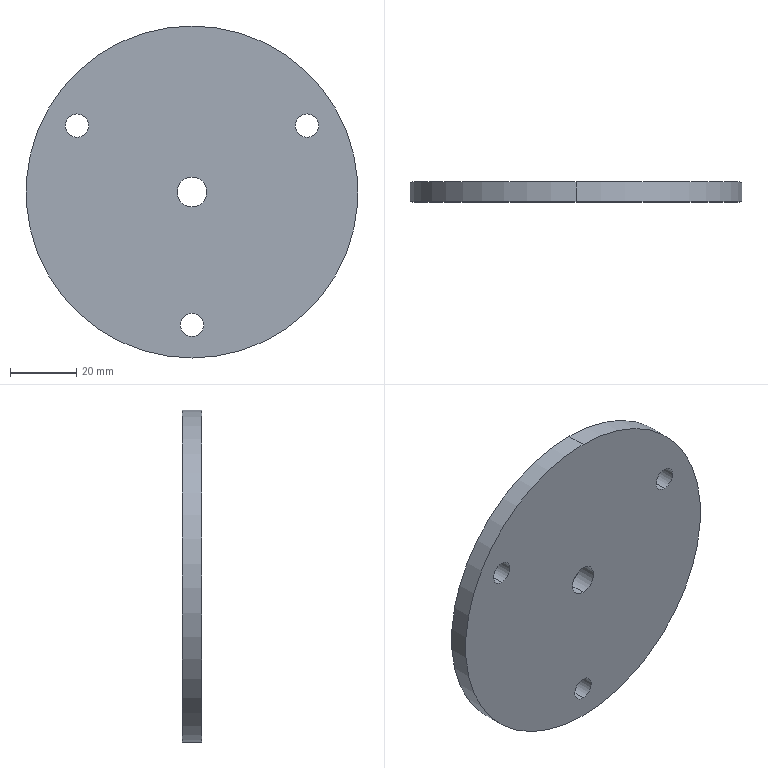Part | SolidWorks | features Extrusion 1, HoleWzd 1, ICE 1 | 1 solid | 12 faces | box 100 x 6 x 100 mm | volume 46049 mm3 | cylinder 10 | plane 2 | commonest cylinder face diameters 7 x6 9 x2 100 x2
STEP:
#1=CARTESIAN_POINT('',(0.,-3.,-4.5));
#2=VERTEX_POINT('',#1);
#3=CARTESIAN_POINT('',(0.,-3.,4.5));
#4=VERTEX_POINT('',#3);
#5=CARTESIAN_POINT('',(0.,-3.,0.));
#6=DIRECTION('',(0.,1.,0.));
#7=DIRECTION('',(0.,0.,1.));
#8=AXIS2_PLACEMENT_3D('',#5,#6,#7);
#9=CIRCLE('',#8,4.5);
#10=EDGE_CURVE('',#2,#4,#9,.T.);
#11=ORIENTED_EDGE('',*,*,#10,.F.);
#12=CARTESIAN_POINT('',(0.,3.,-4.5));
#13=VERTEX_POINT('',#12);
#14=CARTESIAN_POINT('',(0.,3.,-4.5));
#15=DIRECTION('',(0.,1.,0.));
#16=VECTOR('',#15,1000.);
#17=LINE('',#14,#16);
#18=EDGE_CURVE('',#2,#13,#17,.T.);
#19=ORIENTED_EDGE('',*,*,#18,.T.);
#20=CARTESIAN_POINT('',(0.,3.,4.5));
#21=VERTEX_POINT('',#20);
#22=CARTESIAN_POINT('',(0.,3.,0.));
#23=DIRECTION('',(0.,1.,0.));
#24=DIRECTION('',(0.,0.,1.));
#25=AXIS2_PLACEMENT_3D('',#22,#23,#24);
#26=CIRCLE('',#25,4.5);
#27=EDGE_CURVE('',#13,#21,#26,.T.);
#28=ORIENTED_EDGE('',*,*,#27,.T.);
#29=CARTESIAN_POINT('',(0.,3.,4.5));
#30=DIRECTION('',(0.,1.,0.));
#31=VECTOR('',#30,1000.);
#32=LINE('',#29,#31);
#33=EDGE_CURVE('',#4,#21,#32,.T.);
#34=ORIENTED_EDGE('',*,*,#33,.F.);
#35=EDGE_LOOP('',(#11,#19,#28,#34));
#36=FACE_OUTER_BOUND('',#35,.T.);
#37=CARTESIAN_POINT('',(0.,3.,0.));
#38=DIRECTION('',(0.,1.,0.));
#39=DIRECTION('',(0.,0.,1.));
#40=AXIS2_PLACEMENT_3D('',#37,#38,#39);
#41=CYLINDRICAL_SURFACE('',#40,4.5);
#42=ADVANCED_FACE('',(#36),#41,.F.);
#43=CARTESIAN_POINT('',(-34.641,-3.,16.5));
#44=VERTEX_POINT('',#43);
#45=CARTESIAN_POINT('',(-34.641,-3.,23.5));
#46=VERTEX_POINT('',#45);
#47=CARTESIAN_POINT('',(-34.641,-3.,20.));
#48=DIRECTION('',(0.,1.,0.));
#49=DIRECTION('',(0.,0.,1.));
#50=AXIS2_PLACEMENT_3D('',#47,#48,#49);
#51=CIRCLE('',#50,3.5);
#52=EDGE_CURVE('',#44,#46,#51,.T.);
#53=ORIENTED_EDGE('',*,*,#52,.F.);
#54=CARTESIAN_POINT('',(-34.641,3.,16.5));
#55=VERTEX_POINT('',#54);
#56=CARTESIAN_POINT('',(-34.641,-3.,16.5));
#57=DIRECTION('',(0.,1.,0.));
#58=VECTOR('',#57,1000.);
#59=LINE('',#56,#58);
#60=EDGE_CURVE('',#44,#55,#59,.T.);
#61=ORIENTED_EDGE('',*,*,#60,.T.);
#62=CARTESIAN_POINT('',(-34.641,3.,23.5));
#63=VERTEX_POINT('',#62);
#64=CARTESIAN_POINT('',(-34.641,3.,20.));
#65=DIRECTION('',(0.,1.,0.));
#66=DIRECTION('',(0.,0.,1.));
#67=AXIS2_PLACEMENT_3D('',#64,#65,#66);
#68=CIRCLE('',#67,3.5);
#69=EDGE_CURVE('',#55,#63,#68,.T.);
#70=ORIENTED_EDGE('',*,*,#69,.T.);
#71=CARTESIAN_POINT('',(-34.641,-3.,23.5));
#72=DIRECTION('',(0.,1.,0.));
#73=VECTOR('',#72,1000.);
#74=LINE('',#71,#73);
#75=EDGE_CURVE('',#46,#63,#74,.T.);
#76=ORIENTED_EDGE('',*,*,#75,.F.);
#77=EDGE_LOOP('',(#53,#61,#70,#76));
#78=FACE_OUTER_BOUND('',#77,.T.);
#79=CARTESIAN_POINT('',(-34.641,-3.,20.));
#80=DIRECTION('',(0.,1.,0.));
#81=DIRECTION('',(0.,0.,1.));
#82=AXIS2_PLACEMENT_3D('',#79,#80,#81);
#83=CYLINDRICAL_SURFACE('',#82,3.5);
#84=ADVANCED_FACE('',(#78),#83,.F.);
#85=CARTESIAN_POINT('',(34.641,-3.,16.5));
#86=VERTEX_POINT('',#85);
#87=CARTESIAN_POINT('',(34.641,-3.,23.5));
#88=VERTEX_POINT('',#87);
#89=CARTESIAN_POINT('',(34.641,-3.,20.));
#90=DIRECTION('',(0.,1.,0.));
#91=DIRECTION('',(0.,0.,1.));
#92=AXIS2_PLACEMENT_3D('',#89,#90,#91);
#93=CIRCLE('',#92,3.5);
#94=EDGE_CURVE('',#86,#88,#93,.T.);
#95=ORIENTED_EDGE('',*,*,#94,.F.);
#96=CARTESIAN_POINT('',(34.641,3.,16.5));
#97=VERTEX_POINT('',#96);
#98=CARTESIAN_POINT('',(34.641,-3.,16.5));
#99=DIRECTION('',(0.,1.,0.));
#100=VECTOR('',#99,1000.);
#101=LINE('',#98,#100);
#102=EDGE_CURVE('',#86,#97,#101,.T.);
#103=ORIENTED_EDGE('',*,*,#102,.T.);
#104=CARTESIAN_POINT('',(34.641,3.,23.5));
#105=VERTEX_POINT('',#104);
#106=CARTESIAN_POINT('',(34.641,3.,20.));
#107=DIRECTION('',(0.,1.,0.));
#108=DIRECTION('',(0.,0.,1.));
#109=AXIS2_PLACEMENT_3D('',#106,#107,#108);
#110=CIRCLE('',#109,3.5);
#111=EDGE_CURVE('',#97,#105,#110,.T.);
#112=ORIENTED_EDGE('',*,*,#111,.T.);
#113=CARTESIAN_POINT('',(34.641,-3.,23.5));
#114=DIRECTION('',(0.,1.,0.));
#115=VECTOR('',#114,1000.);
#116=LINE('',#113,#115);
#117=EDGE_CURVE('',#88,#105,#116,.T.);
#118=ORIENTED_EDGE('',*,*,#117,.F.);
#119=EDGE_LOOP('',(#95,#103,#112,#118));
#120=FACE_OUTER_BOUND('',#119,.T.);
#121=CARTESIAN_POINT('',(34.641,-3.,20.));
#122=DIRECTION('',(0.,1.,0.));
#123=DIRECTION('',(0.,0.,1.));
#124=AXIS2_PLACEMENT_3D('',#121,#122,#123);
#125=CYLINDRICAL_SURFACE('',#124,3.5);
#126=ADVANCED_FACE('',(#120),#125,.F.);
#127=CARTESIAN_POINT('',(0.,-3.,-43.5));
#128=VERTEX_POINT('',#127);
#129=CARTESIAN_POINT('',(0.,-3.,-36.5));
#130=VERTEX_POINT('',#129);
#131=CARTESIAN_POINT('',(0.,-3.,-40.));
#132=DIRECTION('',(0.,1.,0.));
#133=DIRECTION('',(0.,0.,1.));
#134=AXIS2_PLACEMENT_3D('',#131,#132,#133);
#135=CIRCLE('',#134,3.5);
#136=EDGE_CURVE('',#128,#130,#135,.T.);
#137=ORIENTED_EDGE('',*,*,#136,.F.);
#138=CARTESIAN_POINT('',(0.,3.,-43.5));
#139=VERTEX_POINT('',#138);
#140=CARTESIAN_POINT('',(0.,-3.,-43.5));
#141=DIRECTION('',(0.,1.,0.));
#142=VECTOR('',#141,1000.);
#143=LINE('',#140,#142);
#144=EDGE_CURVE('',#128,#139,#143,.T.);
#145=ORIENTED_EDGE('',*,*,#144,.T.);
#146=CARTESIAN_POINT('',(0.,3.,-36.5));
#147=VERTEX_POINT('',#146);
#148=CARTESIAN_POINT('',(0.,3.,-40.));
#149=DIRECTION('',(0.,1.,0.));
#150=DIRECTION('',(0.,0.,1.));
#151=AXIS2_PLACEMENT_3D('',#148,#149,#150);
#152=CIRCLE('',#151,3.5);
#153=EDGE_CURVE('',#139,#147,#152,.T.);
#154=ORIENTED_EDGE('',*,*,#153,.T.);
#155=CARTESIAN_POINT('',(0.,-3.,-36.5));
#156=DIRECTION('',(0.,1.,0.));
#157=VECTOR('',#156,1000.);
#158=LINE('',#155,#157);
#159=EDGE_CURVE('',#130,#147,#158,.T.);
#160=ORIENTED_EDGE('',*,*,#159,.F.);
#161=EDGE_LOOP('',(#137,#145,#154,#160));
#162=FACE_OUTER_BOUND('',#161,.T.);
#163=CARTESIAN_POINT('',(0.,-3.,-40.));
#164=DIRECTION('',(0.,1.,0.));
#165=DIRECTION('',(0.,0.,1.));
#166=AXIS2_PLACEMENT_3D('',#163,#164,#165);
#167=CYLINDRICAL_SURFACE('',#166,3.5);
#168=ADVANCED_FACE('',(#162),#167,.F.);
#169=CARTESIAN_POINT('',(0.,3.,50.));
#170=VERTEX_POINT('',#169);
#171=CARTESIAN_POINT('',(0.,3.,-50.));
#172=VERTEX_POINT('',#171);
#173=CARTESIAN_POINT('',(0.,3.,0.));
#174=DIRECTION('',(0.,1.,0.));
#175=DIRECTION('',(0.,0.,1.));
#176=AXIS2_PLACEMENT_3D('',#173,#174,#175);
#177=CIRCLE('',#176,50.);
#178=EDGE_CURVE('',#170,#172,#177,.T.);
#179=ORIENTED_EDGE('',*,*,#178,.F.);
#180=CARTESIAN_POINT('',(0.,-3.,50.));
#181=VERTEX_POINT('',#180);
#182=CARTESIAN_POINT('',(0.,3.,50.));
#183=DIRECTION('',(0.,-1.,0.));
#184=VECTOR('',#183,1000.);
#185=LINE('',#182,#184);
#186=EDGE_CURVE('',#170,#181,#185,.T.);
#187=ORIENTED_EDGE('',*,*,#186,.T.);
#188=CARTESIAN_POINT('',(0.,-3.,-50.));
#189=VERTEX_POINT('',#188);
#190=CARTESIAN_POINT('',(0.,-3.,0.));
#191=DIRECTION('',(0.,1.,0.));
#192=DIRECTION('',(0.,0.,1.));
#193=AXIS2_PLACEMENT_3D('',#190,#191,#192);
#194=CIRCLE('',#193,50.);
#195=EDGE_CURVE('',#181,#189,#194,.T.);
#196=ORIENTED_EDGE('',*,*,#195,.T.);
#197=CARTESIAN_POINT('',(0.,3.,-50.));
#198=DIRECTION('',(0.,-1.,0.));
#199=VECTOR('',#198,1000.);
#200=LINE('',#197,#199);
#201=EDGE_CURVE('',#172,#189,#200,.T.);
#202=ORIENTED_EDGE('',*,*,#201,.F.);
#203=EDGE_LOOP('',(#179,#187,#196,#202));
#204=FACE_OUTER_BOUND('',#203,.T.);
#205=CARTESIAN_POINT('',(0.,3.,0.));
#206=DIRECTION('',(0.,-1.,0.));
#207=DIRECTION('',(0.,0.,-1.));
#208=AXIS2_PLACEMENT_3D('',#205,#206,#207);
#209=CYLINDRICAL_SURFACE('',#208,50.);
#210=ADVANCED_FACE('',(#204),#209,.T.);
#211=ORIENTED_EDGE('',*,*,#186,.F.);
#212=CARTESIAN_POINT('',(0.,3.,0.));
#213=DIRECTION('',(0.,1.,0.));
#214=DIRECTION('',(0.,0.,1.));
#215=AXIS2_PLACEMENT_3D('',#212,#213,#214);
#216=CIRCLE('',#215,50.);
#217=EDGE_CURVE('',#172,#170,#216,.T.);
#218=ORIENTED_EDGE('',*,*,#217,.F.);
#219=ORIENTED_EDGE('',*,*,#201,.T.);
#220=CARTESIAN_POINT('',(0.,-3.,0.));
#221=DIRECTION('',(0.,1.,0.));
#222=DIRECTION('',(0.,0.,1.));
#223=AXIS2_PLACEMENT_3D('',#220,#221,#222);
#224=CIRCLE('',#223,50.);
#225=EDGE_CURVE('',#189,#181,#224,.T.);
#226=ORIENTED_EDGE('',*,*,#225,.T.);
#227=EDGE_LOOP('',(#211,#218,#219,#226));
#228=FACE_OUTER_BOUND('',#227,.T.);
#229=CARTESIAN_POINT('',(0.,3.,0.));
#230=DIRECTION('',(0.,-1.,0.));
#231=DIRECTION('',(0.,0.,-1.));
#232=AXIS2_PLACEMENT_3D('',#229,#230,#231);
#233=CYLINDRICAL_SURFACE('',#232,50.);
#234=ADVANCED_FACE('',(#228),#233,.T.);
#235=CARTESIAN_POINT('',(0.,3.,0.));
#236=DIRECTION('',(0.,1.,0.));
#237=DIRECTION('',(0.,0.,1.));
#238=AXIS2_PLACEMENT_3D('',#235,#236,#237);
#239=CIRCLE('',#238,4.5);
#240=EDGE_CURVE('',#21,#13,#239,.T.);
#241=ORIENTED_EDGE('',*,*,#240,.F.);
#242=ORIENTED_EDGE('',*,*,#27,.F.);
#243=EDGE_LOOP('',(#241,#242));
#244=FACE_BOUND('',#243,.T.);
#245=CARTESIAN_POINT('',(-34.641,3.,20.));
#246=DIRECTION('',(0.,1.,0.));
#247=DIRECTION('',(0.,0.,1.));
#248=AXIS2_PLACEMENT_3D('',#245,#246,#247);
#249=CIRCLE('',#248,3.5);
#250=EDGE_CURVE('',#63,#55,#249,.T.);
#251=ORIENTED_EDGE('',*,*,#250,.F.);
#252=ORIENTED_EDGE('',*,*,#69,.F.);
#253=EDGE_LOOP('',(#251,#252));
#254=FACE_BOUND('',#253,.T.);
#255=CARTESIAN_POINT('',(34.641,3.,20.));
#256=DIRECTION('',(0.,1.,0.));
#257=DIRECTION('',(0.,0.,1.));
#258=AXIS2_PLACEMENT_3D('',#255,#256,#257);
#259=CIRCLE('',#258,3.5);
#260=EDGE_CURVE('',#105,#97,#259,.T.);
#261=ORIENTED_EDGE('',*,*,#260,.F.);
#262=ORIENTED_EDGE('',*,*,#111,.F.);
#263=EDGE_LOOP('',(#261,#262));
#264=FACE_BOUND('',#263,.T.);
#265=CARTESIAN_POINT('',(0.,3.,-40.));
#266=DIRECTION('',(0.,1.,0.));
#267=DIRECTION('',(0.,0.,1.));
#268=AXIS2_PLACEMENT_3D('',#265,#266,#267);
#269=CIRCLE('',#268,3.5);
#270=EDGE_CURVE('',#147,#139,#269,.T.);
#271=ORIENTED_EDGE('',*,*,#270,.F.);
#272=ORIENTED_EDGE('',*,*,#153,.F.);
#273=EDGE_LOOP('',(#271,#272));
#274=FACE_BOUND('',#273,.T.);
#275=ORIENTED_EDGE('',*,*,#217,.T.);
#276=ORIENTED_EDGE('',*,*,#178,.T.);
#277=EDGE_LOOP('',(#275,#276));
#278=FACE_OUTER_BOUND('',#277,.T.);
#279=CARTESIAN_POINT('',(0.,3.,0.));
#280=DIRECTION('',(0.,1.,0.));
#281=DIRECTION('',(0.,0.,1.));
#282=AXIS2_PLACEMENT_3D('',#279,#280,#281);
#283=PLANE('',#282);
#284=ADVANCED_FACE('',(#244,#254,#264,#274,#278),#283,.T.);
#285=CARTESIAN_POINT('',(0.,-3.,0.));
#286=DIRECTION('',(0.,1.,0.));
#287=DIRECTION('',(0.,0.,1.));
#288=AXIS2_PLACEMENT_3D('',#285,#286,#287);
#289=CIRCLE('',#288,4.5);
#290=EDGE_CURVE('',#4,#2,#289,.T.);
#291=ORIENTED_EDGE('',*,*,#290,.T.);
#292=ORIENTED_EDGE('',*,*,#10,.T.);
#293=EDGE_LOOP('',(#291,#292));
#294=FACE_BOUND('',#293,.T.);
#295=CARTESIAN_POINT('',(-34.641,-3.,20.));
#296=DIRECTION('',(0.,1.,0.));
#297=DIRECTION('',(0.,0.,1.));
#298=AXIS2_PLACEMENT_3D('',#295,#296,#297);
#299=CIRCLE('',#298,3.5);
#300=EDGE_CURVE('',#46,#44,#299,.T.);
#301=ORIENTED_EDGE('',*,*,#300,.T.);
#302=ORIENTED_EDGE('',*,*,#52,.T.);
#303=EDGE_LOOP('',(#301,#302));
#304=FACE_BOUND('',#303,.T.);
#305=CARTESIAN_POINT('',(34.641,-3.,20.));
#306=DIRECTION('',(0.,1.,0.));
#307=DIRECTION('',(0.,0.,1.));
#308=AXIS2_PLACEMENT_3D('',#305,#306,#307);
#309=CIRCLE('',#308,3.5);
#310=EDGE_CURVE('',#88,#86,#309,.T.);
#311=ORIENTED_EDGE('',*,*,#310,.T.);
#312=ORIENTED_EDGE('',*,*,#94,.T.);
#313=EDGE_LOOP('',(#311,#312));
#314=FACE_BOUND('',#313,.T.);
#315=CARTESIAN_POINT('',(0.,-3.,-40.));
#316=DIRECTION('',(0.,1.,0.));
#317=DIRECTION('',(0.,0.,1.));
#318=AXIS2_PLACEMENT_3D('',#315,#316,#317);
#319=CIRCLE('',#318,3.5);
#320=EDGE_CURVE('',#130,#128,#319,.T.);
#321=ORIENTED_EDGE('',*,*,#320,.T.);
#322=ORIENTED_EDGE('',*,*,#136,.T.);
#323=EDGE_LOOP('',(#321,#322));
#324=FACE_BOUND('',#323,.T.);
#325=ORIENTED_EDGE('',*,*,#225,.F.);
#326=ORIENTED_EDGE('',*,*,#195,.F.);
#327=EDGE_LOOP('',(#325,#326));
#328=FACE_OUTER_BOUND('',#327,.T.);
#329=CARTESIAN_POINT('',(0.,-3.,0.));
#330=DIRECTION('',(0.,1.,0.));
#331=DIRECTION('',(0.,0.,1.));
#332=AXIS2_PLACEMENT_3D('',#329,#330,#331);
#333=PLANE('',#332);
#334=ADVANCED_FACE('',(#294,#304,#314,#324,#328),#333,.F.);
#335=ORIENTED_EDGE('',*,*,#144,.F.);
#336=ORIENTED_EDGE('',*,*,#320,.F.);
#337=ORIENTED_EDGE('',*,*,#159,.T.);
#338=ORIENTED_EDGE('',*,*,#270,.T.);
#339=EDGE_LOOP('',(#335,#336,#337,#338));
#340=FACE_OUTER_BOUND('',#339,.T.);
#341=CARTESIAN_POINT('',(0.,-3.,-40.));
#342=DIRECTION('',(0.,1.,0.));
#343=DIRECTION('',(0.,0.,1.));
#344=AXIS2_PLACEMENT_3D('',#341,#342,#343);
#345=CYLINDRICAL_SURFACE('',#344,3.5);
#346=ADVANCED_FACE('',(#340),#345,.F.);
#347=ORIENTED_EDGE('',*,*,#102,.F.);
#348=ORIENTED_EDGE('',*,*,#310,.F.);
#349=ORIENTED_EDGE('',*,*,#117,.T.);
#350=ORIENTED_EDGE('',*,*,#260,.T.);
#351=EDGE_LOOP('',(#347,#348,#349,#350));
#352=FACE_OUTER_BOUND('',#351,.T.);
#353=CARTESIAN_POINT('',(34.641,-3.,20.));
#354=DIRECTION('',(0.,1.,0.));
#355=DIRECTION('',(0.,0.,1.));
#356=AXIS2_PLACEMENT_3D('',#353,#354,#355);
#357=CYLINDRICAL_SURFACE('',#356,3.5);
#358=ADVANCED_FACE('',(#352),#357,.F.);
#359=ORIENTED_EDGE('',*,*,#60,.F.);
#360=ORIENTED_EDGE('',*,*,#300,.F.);
#361=ORIENTED_EDGE('',*,*,#75,.T.);
#362=ORIENTED_EDGE('',*,*,#250,.T.);
#363=EDGE_LOOP('',(#359,#360,#361,#362));
#364=FACE_OUTER_BOUND('',#363,.T.);
#365=CARTESIAN_POINT('',(-34.641,-3.,20.));
#366=DIRECTION('',(0.,1.,0.));
#367=DIRECTION('',(0.,0.,1.));
#368=AXIS2_PLACEMENT_3D('',#365,#366,#367);
#369=CYLINDRICAL_SURFACE('',#368,3.5);
#370=ADVANCED_FACE('',(#364),#369,.F.);
#371=ORIENTED_EDGE('',*,*,#18,.F.);
#372=ORIENTED_EDGE('',*,*,#290,.F.);
#373=ORIENTED_EDGE('',*,*,#33,.T.);
#374=ORIENTED_EDGE('',*,*,#240,.T.);
#375=EDGE_LOOP('',(#371,#372,#373,#374));
#376=FACE_OUTER_BOUND('',#375,.T.);
#377=CARTESIAN_POINT('',(0.,3.,0.));
#378=DIRECTION('',(0.,1.,0.));
#379=DIRECTION('',(0.,0.,1.));
#380=AXIS2_PLACEMENT_3D('',#377,#378,#379);
#381=CYLINDRICAL_SURFACE('',#380,4.5);
#382=ADVANCED_FACE('',(#376),#381,.F.);
#383=CLOSED_SHELL('',(#42,#84,#126,#168,#210,#234,#284,#334,#346,#358,#370,#382));
#384=MANIFOLD_SOLID_BREP('',#383);
#385=CARTESIAN_POINT('',(0.,0.,0.));
#386=DIRECTION('',(0.,0.,1.));
#387=DIRECTION('',(1.,0.,0.));
#388=AXIS2_PLACEMENT_3D('',#385,#386,#387);
#389=(LENGTH_UNIT()NAMED_UNIT(*)SI_UNIT(.MILLI.,.METRE.));
#390=UNCERTAINTY_MEASURE_WITH_UNIT(LENGTH_MEASURE(0.00001),#389,'','');
#391=(NAMED_UNIT(*)PLANE_ANGLE_UNIT()SI_UNIT($,.RADIAN.));
#392=(NAMED_UNIT(*)SI_UNIT($,.STERADIAN.)SOLID_ANGLE_UNIT());
#393=(GEOMETRIC_REPRESENTATION_CONTEXT(3)GLOBAL_UNCERTAINTY_ASSIGNED_CONTEXT((#390))GLOBAL_UNIT_ASSIGNED_CONTEXT((#389,#391,#392))REPRESENTATION_CONTEXT('',''));
#394=ADVANCED_BREP_SHAPE_REPRESENTATION('',(#384,#388),#393);